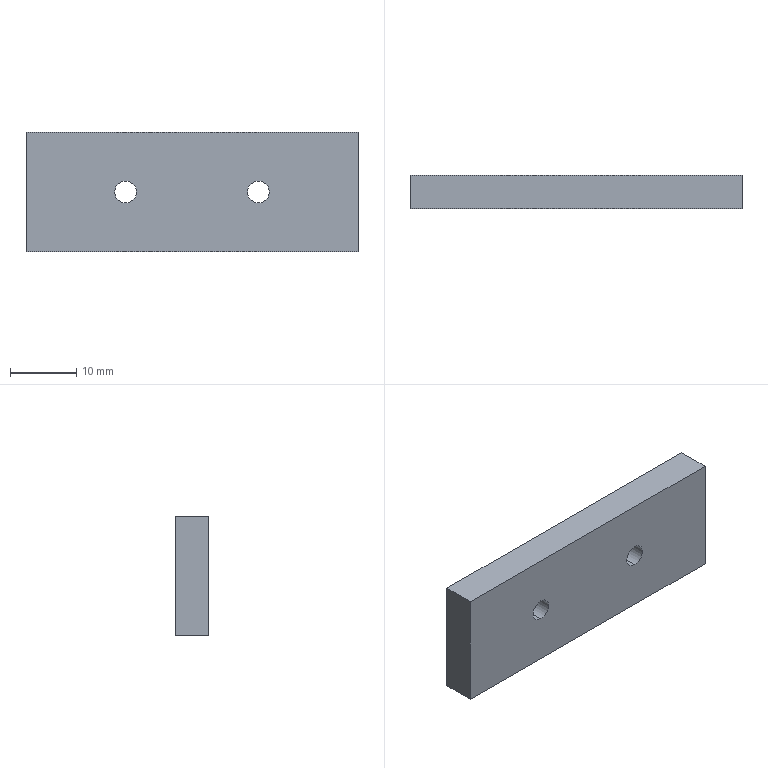Part | SolidWorks | features Extrusion 1, HoleWzd 1 | 1 solid | 10 faces | box 50 x 5 x 18 mm | volume 4414 mm3 | plane 6 | cylinder 4 | commonest cylinder face diameters 3.3 x4
STEP:
#1=CARTESIAN_POINT('',(15.,-2.5,-1.65));
#2=VERTEX_POINT('',#1);
#3=CARTESIAN_POINT('',(15.,-2.5,1.65));
#4=VERTEX_POINT('',#3);
#5=CARTESIAN_POINT('',(15.,-2.5,0.));
#6=DIRECTION('',(0.,1.,0.));
#7=DIRECTION('',(0.,0.,1.));
#8=AXIS2_PLACEMENT_3D('',#5,#6,#7);
#9=CIRCLE('',#8,1.65);
#10=EDGE_CURVE('',#2,#4,#9,.T.);
#11=ORIENTED_EDGE('',*,*,#10,.F.);
#12=CARTESIAN_POINT('',(15.,2.5,-1.65));
#13=VERTEX_POINT('',#12);
#14=CARTESIAN_POINT('',(15.,2.5,-1.65));
#15=DIRECTION('',(0.,1.,0.));
#16=VECTOR('',#15,1000.);
#17=LINE('',#14,#16);
#18=EDGE_CURVE('',#2,#13,#17,.T.);
#19=ORIENTED_EDGE('',*,*,#18,.T.);
#20=CARTESIAN_POINT('',(15.,2.5,1.65));
#21=VERTEX_POINT('',#20);
#22=CARTESIAN_POINT('',(15.,2.5,0.));
#23=DIRECTION('',(0.,1.,0.));
#24=DIRECTION('',(0.,0.,1.));
#25=AXIS2_PLACEMENT_3D('',#22,#23,#24);
#26=CIRCLE('',#25,1.65);
#27=EDGE_CURVE('',#13,#21,#26,.T.);
#28=ORIENTED_EDGE('',*,*,#27,.T.);
#29=CARTESIAN_POINT('',(15.,2.5,1.65));
#30=DIRECTION('',(0.,1.,0.));
#31=VECTOR('',#30,1000.);
#32=LINE('',#29,#31);
#33=EDGE_CURVE('',#4,#21,#32,.T.);
#34=ORIENTED_EDGE('',*,*,#33,.F.);
#35=EDGE_LOOP('',(#11,#19,#28,#34));
#36=FACE_OUTER_BOUND('',#35,.T.);
#37=CARTESIAN_POINT('',(15.,2.5,0.));
#38=DIRECTION('',(0.,1.,0.));
#39=DIRECTION('',(0.,0.,1.));
#40=AXIS2_PLACEMENT_3D('',#37,#38,#39);
#41=CYLINDRICAL_SURFACE('',#40,1.65);
#42=ADVANCED_FACE('',(#36),#41,.F.);
#43=CARTESIAN_POINT('',(35.,-2.5,-1.65));
#44=VERTEX_POINT('',#43);
#45=CARTESIAN_POINT('',(35.,-2.5,1.65));
#46=VERTEX_POINT('',#45);
#47=CARTESIAN_POINT('',(35.,-2.5,0.));
#48=DIRECTION('',(0.,1.,0.));
#49=DIRECTION('',(0.,0.,1.));
#50=AXIS2_PLACEMENT_3D('',#47,#48,#49);
#51=CIRCLE('',#50,1.65);
#52=EDGE_CURVE('',#44,#46,#51,.T.);
#53=ORIENTED_EDGE('',*,*,#52,.F.);
#54=CARTESIAN_POINT('',(35.,2.5,-1.65));
#55=VERTEX_POINT('',#54);
#56=CARTESIAN_POINT('',(35.,2.5,-1.65));
#57=DIRECTION('',(0.,1.,0.));
#58=VECTOR('',#57,1000.);
#59=LINE('',#56,#58);
#60=EDGE_CURVE('',#44,#55,#59,.T.);
#61=ORIENTED_EDGE('',*,*,#60,.T.);
#62=CARTESIAN_POINT('',(35.,2.5,1.65));
#63=VERTEX_POINT('',#62);
#64=CARTESIAN_POINT('',(35.,2.5,0.));
#65=DIRECTION('',(0.,1.,0.));
#66=DIRECTION('',(0.,0.,1.));
#67=AXIS2_PLACEMENT_3D('',#64,#65,#66);
#68=CIRCLE('',#67,1.65);
#69=EDGE_CURVE('',#55,#63,#68,.T.);
#70=ORIENTED_EDGE('',*,*,#69,.T.);
#71=CARTESIAN_POINT('',(35.,2.5,1.65));
#72=DIRECTION('',(0.,1.,0.));
#73=VECTOR('',#72,1000.);
#74=LINE('',#71,#73);
#75=EDGE_CURVE('',#46,#63,#74,.T.);
#76=ORIENTED_EDGE('',*,*,#75,.F.);
#77=EDGE_LOOP('',(#53,#61,#70,#76));
#78=FACE_OUTER_BOUND('',#77,.T.);
#79=CARTESIAN_POINT('',(35.,2.5,0.));
#80=DIRECTION('',(0.,1.,0.));
#81=DIRECTION('',(0.,0.,1.));
#82=AXIS2_PLACEMENT_3D('',#79,#80,#81);
#83=CYLINDRICAL_SURFACE('',#82,1.65);
#84=ADVANCED_FACE('',(#78),#83,.F.);
#85=CARTESIAN_POINT('',(0.,-2.5,-9.));
#86=VERTEX_POINT('',#85);
#87=CARTESIAN_POINT('',(0.,-2.5,9.));
#88=VERTEX_POINT('',#87);
#89=CARTESIAN_POINT('',(0.,-2.5,0.));
#90=DIRECTION('',(0.,0.,1.));
#91=VECTOR('',#90,1000.);
#92=LINE('',#89,#91);
#93=EDGE_CURVE('',#86,#88,#92,.T.);
#94=ORIENTED_EDGE('',*,*,#93,.T.);
#95=CARTESIAN_POINT('',(0.,2.5,9.));
#96=VERTEX_POINT('',#95);
#97=CARTESIAN_POINT('',(0.,2.5,9.));
#98=DIRECTION('',(0.,-1.,0.));
#99=VECTOR('',#98,1000.);
#100=LINE('',#97,#99);
#101=EDGE_CURVE('',#96,#88,#100,.T.);
#102=ORIENTED_EDGE('',*,*,#101,.F.);
#103=CARTESIAN_POINT('',(0.,2.5,-9.));
#104=VERTEX_POINT('',#103);
#105=CARTESIAN_POINT('',(0.,2.5,-9.));
#106=DIRECTION('',(0.,0.,1.));
#107=VECTOR('',#106,1000.);
#108=LINE('',#105,#107);
#109=EDGE_CURVE('',#104,#96,#108,.T.);
#110=ORIENTED_EDGE('',*,*,#109,.F.);
#111=CARTESIAN_POINT('',(0.,2.5,-9.));
#112=DIRECTION('',(0.,-1.,0.));
#113=VECTOR('',#112,1000.);
#114=LINE('',#111,#113);
#115=EDGE_CURVE('',#104,#86,#114,.T.);
#116=ORIENTED_EDGE('',*,*,#115,.T.);
#117=EDGE_LOOP('',(#94,#102,#110,#116));
#118=FACE_OUTER_BOUND('',#117,.T.);
#119=CARTESIAN_POINT('',(0.,2.5,0.));
#120=DIRECTION('',(1.,0.,0.));
#121=DIRECTION('',(0.,0.,-1.));
#122=AXIS2_PLACEMENT_3D('',#119,#120,#121);
#123=PLANE('',#122);
#124=ADVANCED_FACE('',(#118),#123,.F.);
#125=CARTESIAN_POINT('',(50.,-2.5,9.));
#126=VERTEX_POINT('',#125);
#127=CARTESIAN_POINT('',(0.,-2.5,9.));
#128=DIRECTION('',(1.,0.,0.));
#129=VECTOR('',#128,1000.);
#130=LINE('',#127,#129);
#131=EDGE_CURVE('',#88,#126,#130,.T.);
#132=ORIENTED_EDGE('',*,*,#131,.T.);
#133=CARTESIAN_POINT('',(50.,2.5,9.));
#134=VERTEX_POINT('',#133);
#135=CARTESIAN_POINT('',(50.,2.5,9.));
#136=DIRECTION('',(0.,-1.,0.));
#137=VECTOR('',#136,1000.);
#138=LINE('',#135,#137);
#139=EDGE_CURVE('',#134,#126,#138,.T.);
#140=ORIENTED_EDGE('',*,*,#139,.F.);
#141=CARTESIAN_POINT('',(0.,2.5,9.));
#142=DIRECTION('',(1.,0.,0.));
#143=VECTOR('',#142,1000.);
#144=LINE('',#141,#143);
#145=EDGE_CURVE('',#96,#134,#144,.T.);
#146=ORIENTED_EDGE('',*,*,#145,.F.);
#147=ORIENTED_EDGE('',*,*,#101,.T.);
#148=EDGE_LOOP('',(#132,#140,#146,#147));
#149=FACE_OUTER_BOUND('',#148,.T.);
#150=CARTESIAN_POINT('',(0.,2.5,9.));
#151=DIRECTION('',(0.,0.,-1.));
#152=DIRECTION('',(-1.,0.,0.));
#153=AXIS2_PLACEMENT_3D('',#150,#151,#152);
#154=PLANE('',#153);
#155=ADVANCED_FACE('',(#149),#154,.F.);
#156=CARTESIAN_POINT('',(50.,-2.5,-9.));
#157=VERTEX_POINT('',#156);
#158=CARTESIAN_POINT('',(50.,-2.5,9.));
#159=DIRECTION('',(0.,0.,-1.));
#160=VECTOR('',#159,1000.);
#161=LINE('',#158,#160);
#162=EDGE_CURVE('',#126,#157,#161,.T.);
#163=ORIENTED_EDGE('',*,*,#162,.T.);
#164=CARTESIAN_POINT('',(50.,2.5,-9.));
#165=VERTEX_POINT('',#164);
#166=CARTESIAN_POINT('',(50.,2.5,-9.));
#167=DIRECTION('',(0.,-1.,0.));
#168=VECTOR('',#167,1000.);
#169=LINE('',#166,#168);
#170=EDGE_CURVE('',#165,#157,#169,.T.);
#171=ORIENTED_EDGE('',*,*,#170,.F.);
#172=CARTESIAN_POINT('',(50.,2.5,9.));
#173=DIRECTION('',(0.,0.,-1.));
#174=VECTOR('',#173,1000.);
#175=LINE('',#172,#174);
#176=EDGE_CURVE('',#134,#165,#175,.T.);
#177=ORIENTED_EDGE('',*,*,#176,.F.);
#178=ORIENTED_EDGE('',*,*,#139,.T.);
#179=EDGE_LOOP('',(#163,#171,#177,#178));
#180=FACE_OUTER_BOUND('',#179,.T.);
#181=CARTESIAN_POINT('',(50.,2.5,9.));
#182=DIRECTION('',(-1.,0.,0.));
#183=DIRECTION('',(0.,0.,1.));
#184=AXIS2_PLACEMENT_3D('',#181,#182,#183);
#185=PLANE('',#184);
#186=ADVANCED_FACE('',(#180),#185,.F.);
#187=CARTESIAN_POINT('',(50.,-2.5,-9.));
#188=DIRECTION('',(-1.,0.,0.));
#189=VECTOR('',#188,1000.);
#190=LINE('',#187,#189);
#191=EDGE_CURVE('',#157,#86,#190,.T.);
#192=ORIENTED_EDGE('',*,*,#191,.T.);
#193=ORIENTED_EDGE('',*,*,#115,.F.);
#194=CARTESIAN_POINT('',(50.,2.5,-9.));
#195=DIRECTION('',(-1.,0.,0.));
#196=VECTOR('',#195,1000.);
#197=LINE('',#194,#196);
#198=EDGE_CURVE('',#165,#104,#197,.T.);
#199=ORIENTED_EDGE('',*,*,#198,.F.);
#200=ORIENTED_EDGE('',*,*,#170,.T.);
#201=EDGE_LOOP('',(#192,#193,#199,#200));
#202=FACE_OUTER_BOUND('',#201,.T.);
#203=CARTESIAN_POINT('',(50.,2.5,-9.));
#204=DIRECTION('',(0.,0.,1.));
#205=DIRECTION('',(1.,0.,0.));
#206=AXIS2_PLACEMENT_3D('',#203,#204,#205);
#207=PLANE('',#206);
#208=ADVANCED_FACE('',(#202),#207,.F.);
#209=CARTESIAN_POINT('',(15.,2.5,0.));
#210=DIRECTION('',(0.,1.,0.));
#211=DIRECTION('',(0.,0.,1.));
#212=AXIS2_PLACEMENT_3D('',#209,#210,#211);
#213=CIRCLE('',#212,1.65);
#214=EDGE_CURVE('',#21,#13,#213,.T.);
#215=ORIENTED_EDGE('',*,*,#214,.F.);
#216=ORIENTED_EDGE('',*,*,#27,.F.);
#217=EDGE_LOOP('',(#215,#216));
#218=FACE_BOUND('',#217,.T.);
#219=CARTESIAN_POINT('',(35.,2.5,0.));
#220=DIRECTION('',(0.,1.,0.));
#221=DIRECTION('',(0.,0.,1.));
#222=AXIS2_PLACEMENT_3D('',#219,#220,#221);
#223=CIRCLE('',#222,1.65);
#224=EDGE_CURVE('',#63,#55,#223,.T.);
#225=ORIENTED_EDGE('',*,*,#224,.F.);
#226=ORIENTED_EDGE('',*,*,#69,.F.);
#227=EDGE_LOOP('',(#225,#226));
#228=FACE_BOUND('',#227,.T.);
#229=ORIENTED_EDGE('',*,*,#109,.T.);
#230=ORIENTED_EDGE('',*,*,#145,.T.);
#231=ORIENTED_EDGE('',*,*,#176,.T.);
#232=ORIENTED_EDGE('',*,*,#198,.T.);
#233=EDGE_LOOP('',(#229,#230,#231,#232));
#234=FACE_OUTER_BOUND('',#233,.T.);
#235=CARTESIAN_POINT('',(0.,2.5,0.));
#236=DIRECTION('',(0.,1.,0.));
#237=DIRECTION('',(0.,0.,1.));
#238=AXIS2_PLACEMENT_3D('',#235,#236,#237);
#239=PLANE('',#238);
#240=ADVANCED_FACE('',(#218,#228,#234),#239,.T.);
#241=CARTESIAN_POINT('',(15.,-2.5,0.));
#242=DIRECTION('',(0.,1.,0.));
#243=DIRECTION('',(0.,0.,1.));
#244=AXIS2_PLACEMENT_3D('',#241,#242,#243);
#245=CIRCLE('',#244,1.65);
#246=EDGE_CURVE('',#4,#2,#245,.T.);
#247=ORIENTED_EDGE('',*,*,#246,.T.);
#248=ORIENTED_EDGE('',*,*,#10,.T.);
#249=EDGE_LOOP('',(#247,#248));
#250=FACE_BOUND('',#249,.T.);
#251=CARTESIAN_POINT('',(35.,-2.5,0.));
#252=DIRECTION('',(0.,1.,0.));
#253=DIRECTION('',(0.,0.,1.));
#254=AXIS2_PLACEMENT_3D('',#251,#252,#253);
#255=CIRCLE('',#254,1.65);
#256=EDGE_CURVE('',#46,#44,#255,.T.);
#257=ORIENTED_EDGE('',*,*,#256,.T.);
#258=ORIENTED_EDGE('',*,*,#52,.T.);
#259=EDGE_LOOP('',(#257,#258));
#260=FACE_BOUND('',#259,.T.);
#261=ORIENTED_EDGE('',*,*,#93,.F.);
#262=ORIENTED_EDGE('',*,*,#191,.F.);
#263=ORIENTED_EDGE('',*,*,#162,.F.);
#264=ORIENTED_EDGE('',*,*,#131,.F.);
#265=EDGE_LOOP('',(#261,#262,#263,#264));
#266=FACE_OUTER_BOUND('',#265,.T.);
#267=CARTESIAN_POINT('',(0.,-2.5,0.));
#268=DIRECTION('',(0.,1.,0.));
#269=DIRECTION('',(0.,0.,1.));
#270=AXIS2_PLACEMENT_3D('',#267,#268,#269);
#271=PLANE('',#270);
#272=ADVANCED_FACE('',(#250,#260,#266),#271,.F.);
#273=ORIENTED_EDGE('',*,*,#60,.F.);
#274=ORIENTED_EDGE('',*,*,#256,.F.);
#275=ORIENTED_EDGE('',*,*,#75,.T.);
#276=ORIENTED_EDGE('',*,*,#224,.T.);
#277=EDGE_LOOP('',(#273,#274,#275,#276));
#278=FACE_OUTER_BOUND('',#277,.T.);
#279=CARTESIAN_POINT('',(35.,2.5,0.));
#280=DIRECTION('',(0.,1.,0.));
#281=DIRECTION('',(0.,0.,1.));
#282=AXIS2_PLACEMENT_3D('',#279,#280,#281);
#283=CYLINDRICAL_SURFACE('',#282,1.65);
#284=ADVANCED_FACE('',(#278),#283,.F.);
#285=ORIENTED_EDGE('',*,*,#18,.F.);
#286=ORIENTED_EDGE('',*,*,#246,.F.);
#287=ORIENTED_EDGE('',*,*,#33,.T.);
#288=ORIENTED_EDGE('',*,*,#214,.T.);
#289=EDGE_LOOP('',(#285,#286,#287,#288));
#290=FACE_OUTER_BOUND('',#289,.T.);
#291=CARTESIAN_POINT('',(15.,2.5,0.));
#292=DIRECTION('',(0.,1.,0.));
#293=DIRECTION('',(0.,0.,1.));
#294=AXIS2_PLACEMENT_3D('',#291,#292,#293);
#295=CYLINDRICAL_SURFACE('',#294,1.65);
#296=ADVANCED_FACE('',(#290),#295,.F.);
#297=CLOSED_SHELL('',(#42,#84,#124,#155,#186,#208,#240,#272,#284,#296));
#298=MANIFOLD_SOLID_BREP('',#297);
#299=CARTESIAN_POINT('',(0.,0.,0.));
#300=DIRECTION('',(0.,0.,1.));
#301=DIRECTION('',(1.,0.,0.));
#302=AXIS2_PLACEMENT_3D('',#299,#300,#301);
#303=(LENGTH_UNIT()NAMED_UNIT(*)SI_UNIT(.MILLI.,.METRE.));
#304=UNCERTAINTY_MEASURE_WITH_UNIT(LENGTH_MEASURE(0.00001),#303,'','');
#305=(NAMED_UNIT(*)PLANE_ANGLE_UNIT()SI_UNIT($,.RADIAN.));
#306=(NAMED_UNIT(*)SI_UNIT($,.STERADIAN.)SOLID_ANGLE_UNIT());
#307=(GEOMETRIC_REPRESENTATION_CONTEXT(3)GLOBAL_UNCERTAINTY_ASSIGNED_CONTEXT((#304))GLOBAL_UNIT_ASSIGNED_CONTEXT((#303,#305,#306))REPRESENTATION_CONTEXT('',''));
#308=ADVANCED_BREP_SHAPE_REPRESENTATION('',(#298,#302),#307);